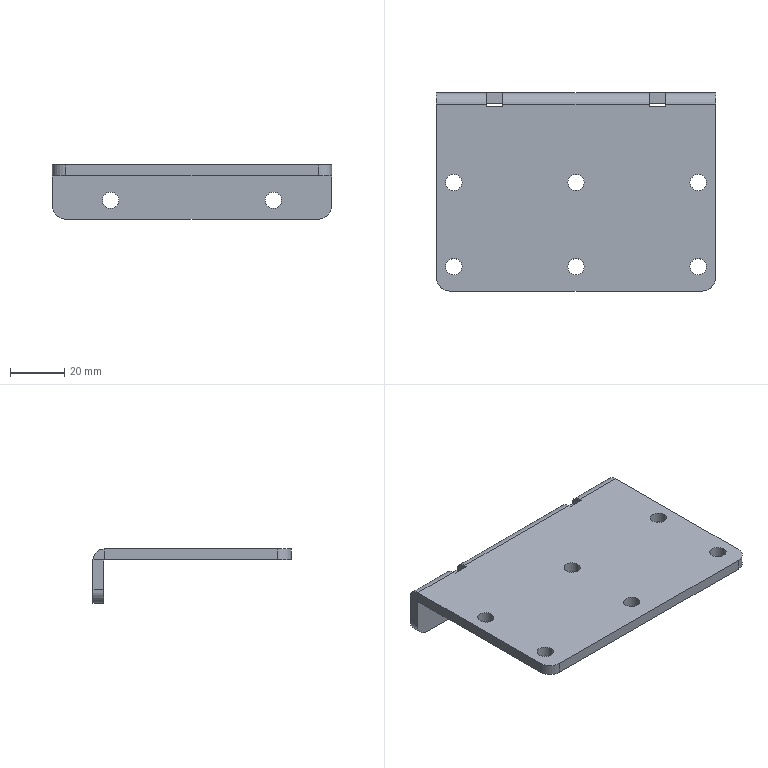Part | SolidWorks | features ICE 3, EdgeFlange 1, Fillet 1, FlatPattern 1, SMBaseFlange 1, SheetMetal 1 | 1 solid | 48 faces | box 103 x 73 x 20 mm | volume 35104 mm3 | cylinder 26 | plane 22 | commonest cylinder face diameters 6 x16 10 x4 0.2 x3 8.2 x3
STEP:
#1=CARTESIAN_POINT('',(-3.,3.5,-4.));
#2=VERTEX_POINT('',#1);
#3=CARTESIAN_POINT('',(3.,3.5,-4.));
#4=VERTEX_POINT('',#3);
#5=CARTESIAN_POINT('',(0.,3.5,-4.));
#6=DIRECTION('',(0.,0.,1.));
#7=DIRECTION('',(1.,0.,0.));
#8=AXIS2_PLACEMENT_3D('',#5,#6,#7);
#9=CIRCLE('',#8,3.);
#10=EDGE_CURVE('',#2,#4,#9,.T.);
#11=ORIENTED_EDGE('',*,*,#10,.F.);
#12=CARTESIAN_POINT('',(-3.,3.5,0.));
#13=VERTEX_POINT('',#12);
#14=CARTESIAN_POINT('',(-3.,3.5,-10.));
#15=DIRECTION('',(0.,0.,1.));
#16=VECTOR('',#15,1000.);
#17=LINE('',#14,#16);
#18=EDGE_CURVE('',#2,#13,#17,.T.);
#19=ORIENTED_EDGE('',*,*,#18,.T.);
#20=CARTESIAN_POINT('',(3.,3.5,0.));
#21=VERTEX_POINT('',#20);
#22=CARTESIAN_POINT('',(0.,3.5,0.));
#23=DIRECTION('',(0.,0.,1.));
#24=DIRECTION('',(1.,0.,0.));
#25=AXIS2_PLACEMENT_3D('',#22,#23,#24);
#26=CIRCLE('',#25,3.);
#27=EDGE_CURVE('',#13,#21,#26,.T.);
#28=ORIENTED_EDGE('',*,*,#27,.T.);
#29=CARTESIAN_POINT('',(3.,3.5,-10.));
#30=DIRECTION('',(0.,0.,1.));
#31=VECTOR('',#30,1000.);
#32=LINE('',#29,#31);
#33=EDGE_CURVE('',#4,#21,#32,.T.);
#34=ORIENTED_EDGE('',*,*,#33,.F.);
#35=EDGE_LOOP('',(#11,#19,#28,#34));
#36=FACE_OUTER_BOUND('',#35,.T.);
#37=CARTESIAN_POINT('',(0.,3.5,-10.));
#38=DIRECTION('',(0.,0.,1.));
#39=DIRECTION('',(1.,0.,0.));
#40=AXIS2_PLACEMENT_3D('',#37,#38,#39);
#41=CYLINDRICAL_SURFACE('',#40,3.);
#42=ADVANCED_FACE('',(#36),#41,.F.);
#43=CARTESIAN_POINT('',(42.,3.5,-4.));
#44=VERTEX_POINT('',#43);
#45=CARTESIAN_POINT('',(48.,3.5,-4.));
#46=VERTEX_POINT('',#45);
#47=CARTESIAN_POINT('',(45.,3.5,-4.));
#48=DIRECTION('',(0.,0.,1.));
#49=DIRECTION('',(1.,0.,0.));
#50=AXIS2_PLACEMENT_3D('',#47,#48,#49);
#51=CIRCLE('',#50,3.);
#52=EDGE_CURVE('',#44,#46,#51,.T.);
#53=ORIENTED_EDGE('',*,*,#52,.F.);
#54=CARTESIAN_POINT('',(42.,3.5,0.));
#55=VERTEX_POINT('',#54);
#56=CARTESIAN_POINT('',(42.,3.5,-10.));
#57=DIRECTION('',(0.,0.,1.));
#58=VECTOR('',#57,1000.);
#59=LINE('',#56,#58);
#60=EDGE_CURVE('',#44,#55,#59,.T.);
#61=ORIENTED_EDGE('',*,*,#60,.T.);
#62=CARTESIAN_POINT('',(48.,3.5,0.));
#63=VERTEX_POINT('',#62);
#64=CARTESIAN_POINT('',(45.,3.5,0.));
#65=DIRECTION('',(0.,0.,1.));
#66=DIRECTION('',(-1.,0.,0.));
#67=AXIS2_PLACEMENT_3D('',#64,#65,#66);
#68=CIRCLE('',#67,3.);
#69=EDGE_CURVE('',#55,#63,#68,.T.);
#70=ORIENTED_EDGE('',*,*,#69,.T.);
#71=CARTESIAN_POINT('',(48.,3.5,-10.));
#72=DIRECTION('',(0.,0.,1.));
#73=VECTOR('',#72,1000.);
#74=LINE('',#71,#73);
#75=EDGE_CURVE('',#46,#63,#74,.T.);
#76=ORIENTED_EDGE('',*,*,#75,.F.);
#77=EDGE_LOOP('',(#53,#61,#70,#76));
#78=FACE_OUTER_BOUND('',#77,.T.);
#79=CARTESIAN_POINT('',(45.,3.5,-10.));
#80=DIRECTION('',(0.,0.,1.));
#81=DIRECTION('',(1.,0.,0.));
#82=AXIS2_PLACEMENT_3D('',#79,#80,#81);
#83=CYLINDRICAL_SURFACE('',#82,3.);
#84=ADVANCED_FACE('',(#78),#83,.F.);
#85=CARTESIAN_POINT('',(42.,-27.5,-4.));
#86=VERTEX_POINT('',#85);
#87=CARTESIAN_POINT('',(48.,-27.5,-4.));
#88=VERTEX_POINT('',#87);
#89=CARTESIAN_POINT('',(45.,-27.5,-4.));
#90=DIRECTION('',(0.,0.,1.));
#91=DIRECTION('',(1.,0.,0.));
#92=AXIS2_PLACEMENT_3D('',#89,#90,#91);
#93=CIRCLE('',#92,3.);
#94=EDGE_CURVE('',#86,#88,#93,.T.);
#95=ORIENTED_EDGE('',*,*,#94,.F.);
#96=CARTESIAN_POINT('',(42.,-27.5,0.));
#97=VERTEX_POINT('',#96);
#98=CARTESIAN_POINT('',(42.,-27.5,-10.));
#99=DIRECTION('',(0.,0.,1.));
#100=VECTOR('',#99,1000.);
#101=LINE('',#98,#100);
#102=EDGE_CURVE('',#86,#97,#101,.T.);
#103=ORIENTED_EDGE('',*,*,#102,.T.);
#104=CARTESIAN_POINT('',(48.,-27.5,0.));
#105=VERTEX_POINT('',#104);
#106=CARTESIAN_POINT('',(45.,-27.5,0.));
#107=DIRECTION('',(0.,0.,1.));
#108=DIRECTION('',(-1.,0.,0.));
#109=AXIS2_PLACEMENT_3D('',#106,#107,#108);
#110=CIRCLE('',#109,3.);
#111=EDGE_CURVE('',#97,#105,#110,.T.);
#112=ORIENTED_EDGE('',*,*,#111,.T.);
#113=CARTESIAN_POINT('',(48.,-27.5,-10.));
#114=DIRECTION('',(0.,0.,1.));
#115=VECTOR('',#114,1000.);
#116=LINE('',#113,#115);
#117=EDGE_CURVE('',#88,#105,#116,.T.);
#118=ORIENTED_EDGE('',*,*,#117,.F.);
#119=EDGE_LOOP('',(#95,#103,#112,#118));
#120=FACE_OUTER_BOUND('',#119,.T.);
#121=CARTESIAN_POINT('',(45.,-27.5,-10.));
#122=DIRECTION('',(0.,0.,1.));
#123=DIRECTION('',(1.,0.,0.));
#124=AXIS2_PLACEMENT_3D('',#121,#122,#123);
#125=CYLINDRICAL_SURFACE('',#124,3.);
#126=ADVANCED_FACE('',(#120),#125,.F.);
#127=CARTESIAN_POINT('',(-48.,3.5,-4.));
#128=VERTEX_POINT('',#127);
#129=CARTESIAN_POINT('',(-42.,3.5,-4.));
#130=VERTEX_POINT('',#129);
#131=CARTESIAN_POINT('',(-45.,3.5,-4.));
#132=DIRECTION('',(0.,0.,1.));
#133=DIRECTION('',(1.,0.,0.));
#134=AXIS2_PLACEMENT_3D('',#131,#132,#133);
#135=CIRCLE('',#134,3.);
#136=EDGE_CURVE('',#128,#130,#135,.T.);
#137=ORIENTED_EDGE('',*,*,#136,.F.);
#138=CARTESIAN_POINT('',(-48.,3.5,0.));
#139=VERTEX_POINT('',#138);
#140=CARTESIAN_POINT('',(-48.,3.5,-10.));
#141=DIRECTION('',(0.,0.,1.));
#142=VECTOR('',#141,1000.);
#143=LINE('',#140,#142);
#144=EDGE_CURVE('',#128,#139,#143,.T.);
#145=ORIENTED_EDGE('',*,*,#144,.T.);
#146=CARTESIAN_POINT('',(-42.,3.5,0.));
#147=VERTEX_POINT('',#146);
#148=CARTESIAN_POINT('',(-45.,3.5,0.));
#149=DIRECTION('',(0.,0.,1.));
#150=DIRECTION('',(1.,0.,0.));
#151=AXIS2_PLACEMENT_3D('',#148,#149,#150);
#152=CIRCLE('',#151,3.);
#153=EDGE_CURVE('',#139,#147,#152,.T.);
#154=ORIENTED_EDGE('',*,*,#153,.T.);
#155=CARTESIAN_POINT('',(-42.,3.5,-10.));
#156=DIRECTION('',(0.,0.,1.));
#157=VECTOR('',#156,1000.);
#158=LINE('',#155,#157);
#159=EDGE_CURVE('',#130,#147,#158,.T.);
#160=ORIENTED_EDGE('',*,*,#159,.F.);
#161=EDGE_LOOP('',(#137,#145,#154,#160));
#162=FACE_OUTER_BOUND('',#161,.T.);
#163=CARTESIAN_POINT('',(-45.,3.5,-10.));
#164=DIRECTION('',(0.,0.,1.));
#165=DIRECTION('',(1.,0.,0.));
#166=AXIS2_PLACEMENT_3D('',#163,#164,#165);
#167=CYLINDRICAL_SURFACE('',#166,3.);
#168=ADVANCED_FACE('',(#162),#167,.F.);
#169=CARTESIAN_POINT('',(-3.,-27.5,-4.));
#170=VERTEX_POINT('',#169);
#171=CARTESIAN_POINT('',(3.,-27.5,-4.));
#172=VERTEX_POINT('',#171);
#173=CARTESIAN_POINT('',(0.,-27.5,-4.));
#174=DIRECTION('',(0.,0.,1.));
#175=DIRECTION('',(1.,0.,0.));
#176=AXIS2_PLACEMENT_3D('',#173,#174,#175);
#177=CIRCLE('',#176,3.);
#178=EDGE_CURVE('',#170,#172,#177,.T.);
#179=ORIENTED_EDGE('',*,*,#178,.F.);
#180=CARTESIAN_POINT('',(-3.,-27.5,0.));
#181=VERTEX_POINT('',#180);
#182=CARTESIAN_POINT('',(-3.,-27.5,-10.));
#183=DIRECTION('',(0.,0.,1.));
#184=VECTOR('',#183,1000.);
#185=LINE('',#182,#184);
#186=EDGE_CURVE('',#170,#181,#185,.T.);
#187=ORIENTED_EDGE('',*,*,#186,.T.);
#188=CARTESIAN_POINT('',(3.,-27.5,0.));
#189=VERTEX_POINT('',#188);
#190=CARTESIAN_POINT('',(0.,-27.5,0.));
#191=DIRECTION('',(0.,0.,1.));
#192=DIRECTION('',(1.,0.,0.));
#193=AXIS2_PLACEMENT_3D('',#190,#191,#192);
#194=CIRCLE('',#193,3.);
#195=EDGE_CURVE('',#181,#189,#194,.T.);
#196=ORIENTED_EDGE('',*,*,#195,.T.);
#197=CARTESIAN_POINT('',(3.,-27.5,-10.));
#198=DIRECTION('',(0.,0.,1.));
#199=VECTOR('',#198,1000.);
#200=LINE('',#197,#199);
#201=EDGE_CURVE('',#172,#189,#200,.T.);
#202=ORIENTED_EDGE('',*,*,#201,.F.);
#203=EDGE_LOOP('',(#179,#187,#196,#202));
#204=FACE_OUTER_BOUND('',#203,.T.);
#205=CARTESIAN_POINT('',(0.,-27.5,-10.));
#206=DIRECTION('',(0.,0.,1.));
#207=DIRECTION('',(1.,0.,0.));
#208=AXIS2_PLACEMENT_3D('',#205,#206,#207);
#209=CYLINDRICAL_SURFACE('',#208,3.);
#210=ADVANCED_FACE('',(#204),#209,.F.);
#211=CARTESIAN_POINT('',(-48.,-27.5,-4.));
#212=VERTEX_POINT('',#211);
#213=CARTESIAN_POINT('',(-42.,-27.5,-4.));
#214=VERTEX_POINT('',#213);
#215=CARTESIAN_POINT('',(-45.,-27.5,-4.));
#216=DIRECTION('',(0.,0.,1.));
#217=DIRECTION('',(1.,0.,0.));
#218=AXIS2_PLACEMENT_3D('',#215,#216,#217);
#219=CIRCLE('',#218,3.);
#220=EDGE_CURVE('',#212,#214,#219,.T.);
#221=ORIENTED_EDGE('',*,*,#220,.F.);
#222=CARTESIAN_POINT('',(-48.,-27.5,0.));
#223=VERTEX_POINT('',#222);
#224=CARTESIAN_POINT('',(-48.,-27.5,-10.));
#225=DIRECTION('',(0.,0.,1.));
#226=VECTOR('',#225,1000.);
#227=LINE('',#224,#226);
#228=EDGE_CURVE('',#212,#223,#227,.T.);
#229=ORIENTED_EDGE('',*,*,#228,.T.);
#230=CARTESIAN_POINT('',(-42.,-27.5,0.));
#231=VERTEX_POINT('',#230);
#232=CARTESIAN_POINT('',(-45.,-27.5,0.));
#233=DIRECTION('',(0.,0.,1.));
#234=DIRECTION('',(1.,0.,0.));
#235=AXIS2_PLACEMENT_3D('',#232,#233,#234);
#236=CIRCLE('',#235,3.);
#237=EDGE_CURVE('',#223,#231,#236,.T.);
#238=ORIENTED_EDGE('',*,*,#237,.T.);
#239=CARTESIAN_POINT('',(-42.,-27.5,-10.));
#240=DIRECTION('',(0.,0.,1.));
#241=VECTOR('',#240,1000.);
#242=LINE('',#239,#241);
#243=EDGE_CURVE('',#214,#231,#242,.T.);
#244=ORIENTED_EDGE('',*,*,#243,.F.);
#245=EDGE_LOOP('',(#221,#229,#238,#244));
#246=FACE_OUTER_BOUND('',#245,.T.);
#247=CARTESIAN_POINT('',(-45.,-27.5,-10.));
#248=DIRECTION('',(0.,0.,1.));
#249=DIRECTION('',(1.,0.,0.));
#250=AXIS2_PLACEMENT_3D('',#247,#248,#249);
#251=CYLINDRICAL_SURFACE('',#250,3.);
#252=ADVANCED_FACE('',(#246),#251,.F.);
#253=CARTESIAN_POINT('',(-30.,32.5,-16.));
#254=VERTEX_POINT('',#253);
#255=CARTESIAN_POINT('',(-30.,32.5,-10.));
#256=VERTEX_POINT('',#255);
#257=CARTESIAN_POINT('',(-30.,32.5,-13.));
#258=DIRECTION('',(0.,1.,0.));
#259=DIRECTION('',(0.,0.,1.));
#260=AXIS2_PLACEMENT_3D('',#257,#258,#259);
#261=CIRCLE('',#260,3.);
#262=EDGE_CURVE('',#254,#256,#261,.T.);
#263=ORIENTED_EDGE('',*,*,#262,.F.);
#264=CARTESIAN_POINT('',(-30.,36.5,-16.));
#265=VERTEX_POINT('',#264);
#266=CARTESIAN_POINT('',(-30.,26.5,-16.));
#267=DIRECTION('',(0.,1.,0.));
#268=VECTOR('',#267,1000.);
#269=LINE('',#266,#268);
#270=EDGE_CURVE('',#254,#265,#269,.T.);
#271=ORIENTED_EDGE('',*,*,#270,.T.);
#272=CARTESIAN_POINT('',(-30.,36.5,-10.));
#273=VERTEX_POINT('',#272);
#274=CARTESIAN_POINT('',(-30.,36.5,-13.));
#275=DIRECTION('',(0.,1.,0.));
#276=DIRECTION('',(0.,0.,1.));
#277=AXIS2_PLACEMENT_3D('',#274,#275,#276);
#278=CIRCLE('',#277,3.);
#279=EDGE_CURVE('',#265,#273,#278,.T.);
#280=ORIENTED_EDGE('',*,*,#279,.T.);
#281=CARTESIAN_POINT('',(-30.,26.5,-10.));
#282=DIRECTION('',(0.,1.,0.));
#283=VECTOR('',#282,1000.);
#284=LINE('',#281,#283);
#285=EDGE_CURVE('',#256,#273,#284,.T.);
#286=ORIENTED_EDGE('',*,*,#285,.F.);
#287=EDGE_LOOP('',(#263,#271,#280,#286));
#288=FACE_OUTER_BOUND('',#287,.T.);
#289=CARTESIAN_POINT('',(-30.,26.5,-13.));
#290=DIRECTION('',(0.,1.,0.));
#291=DIRECTION('',(0.,0.,1.));
#292=AXIS2_PLACEMENT_3D('',#289,#290,#291);
#293=CYLINDRICAL_SURFACE('',#292,3.);
#294=ADVANCED_FACE('',(#288),#293,.F.);
#295=CARTESIAN_POINT('',(30.,32.5,-16.));
#296=VERTEX_POINT('',#295);
#297=CARTESIAN_POINT('',(30.,32.5,-10.));
#298=VERTEX_POINT('',#297);
#299=CARTESIAN_POINT('',(30.,32.5,-13.));
#300=DIRECTION('',(0.,1.,0.));
#301=DIRECTION('',(0.,0.,1.));
#302=AXIS2_PLACEMENT_3D('',#299,#300,#301);
#303=CIRCLE('',#302,3.);
#304=EDGE_CURVE('',#296,#298,#303,.T.);
#305=ORIENTED_EDGE('',*,*,#304,.F.);
#306=CARTESIAN_POINT('',(30.,36.5,-16.));
#307=VERTEX_POINT('',#306);
#308=CARTESIAN_POINT('',(30.,26.5,-16.));
#309=DIRECTION('',(0.,1.,0.));
#310=VECTOR('',#309,1000.);
#311=LINE('',#308,#310);
#312=EDGE_CURVE('',#296,#307,#311,.T.);
#313=ORIENTED_EDGE('',*,*,#312,.T.);
#314=CARTESIAN_POINT('',(30.,36.5,-10.));
#315=VERTEX_POINT('',#314);
#316=CARTESIAN_POINT('',(30.,36.5,-13.));
#317=DIRECTION('',(0.,1.,0.));
#318=DIRECTION('',(0.,0.,-1.));
#319=AXIS2_PLACEMENT_3D('',#316,#317,#318);
#320=CIRCLE('',#319,3.);
#321=EDGE_CURVE('',#307,#315,#320,.T.);
#322=ORIENTED_EDGE('',*,*,#321,.T.);
#323=CARTESIAN_POINT('',(30.,26.5,-10.));
#324=DIRECTION('',(0.,1.,0.));
#325=VECTOR('',#324,1000.);
#326=LINE('',#323,#325);
#327=EDGE_CURVE('',#298,#315,#326,.T.);
#328=ORIENTED_EDGE('',*,*,#327,.F.);
#329=EDGE_LOOP('',(#305,#313,#322,#328));
#330=FACE_OUTER_BOUND('',#329,.T.);
#331=CARTESIAN_POINT('',(30.,26.5,-13.));
#332=DIRECTION('',(0.,1.,0.));
#333=DIRECTION('',(0.,0.,1.));
#334=AXIS2_PLACEMENT_3D('',#331,#332,#333);
#335=CYLINDRICAL_SURFACE('',#334,3.);
#336=ADVANCED_FACE('',(#330),#335,.F.);
#337=CARTESIAN_POINT('',(-27.,31.5,0.));
#338=VERTEX_POINT('',#337);
#339=CARTESIAN_POINT('',(-27.,32.4,0.));
#340=VERTEX_POINT('',#339);
#341=CARTESIAN_POINT('',(-27.,31.5,0.));
#342=DIRECTION('',(0.,1.,0.));
#343=VECTOR('',#342,1000.);
#344=LINE('',#341,#343);
#345=EDGE_CURVE('',#338,#340,#344,.T.);
#346=ORIENTED_EDGE('',*,*,#345,.T.);
#347=CARTESIAN_POINT('',(-27.,32.4,-4.));
#348=VERTEX_POINT('',#347);
#349=CARTESIAN_POINT('',(-27.,32.4,0.));
#350=DIRECTION('',(0.,0.,-1.));
#351=VECTOR('',#350,1000.);
#352=LINE('',#349,#351);
#353=EDGE_CURVE('',#340,#348,#352,.T.);
#354=ORIENTED_EDGE('',*,*,#353,.T.);
#355=CARTESIAN_POINT('',(-27.,31.5,-4.));
#356=VERTEX_POINT('',#355);
#357=CARTESIAN_POINT('',(-27.,0.,-4.));
#358=DIRECTION('',(0.,1.,0.));
#359=VECTOR('',#358,1000.);
#360=LINE('',#357,#359);
#361=EDGE_CURVE('',#356,#348,#360,.T.);
#362=ORIENTED_EDGE('',*,*,#361,.F.);
#363=CARTESIAN_POINT('',(-27.,31.5,-4.1));
#364=DIRECTION('',(0.,0.,-1.));
#365=VECTOR('',#364,1000.);
#366=LINE('',#363,#365);
#367=EDGE_CURVE('',#338,#356,#366,.T.);
#368=ORIENTED_EDGE('',*,*,#367,.F.);
#369=EDGE_LOOP('',(#346,#354,#362,#368));
#370=FACE_OUTER_BOUND('',#369,.T.);
#371=CARTESIAN_POINT('',(-27.,31.5,-4.1));
#372=DIRECTION('',(1.,0.,0.));
#373=DIRECTION('',(0.,0.,-1.));
#374=AXIS2_PLACEMENT_3D('',#371,#372,#373);
#375=PLANE('',#374);
#376=ADVANCED_FACE('',(#370),#375,.F.);
#377=CARTESIAN_POINT('',(33.,31.5,0.));
#378=VERTEX_POINT('',#377);
#379=CARTESIAN_POINT('',(33.,32.4,0.));
#380=VERTEX_POINT('',#379);
#381=CARTESIAN_POINT('',(33.,31.5,0.));
#382=DIRECTION('',(0.,1.,0.));
#383=VECTOR('',#382,1000.);
#384=LINE('',#381,#383);
#385=EDGE_CURVE('',#378,#380,#384,.T.);
#386=ORIENTED_EDGE('',*,*,#385,.T.);
#387=CARTESIAN_POINT('',(33.,32.4,-4.));
#388=VERTEX_POINT('',#387);
#389=CARTESIAN_POINT('',(33.,32.4,0.));
#390=DIRECTION('',(0.,0.,-1.));
#391=VECTOR('',#390,1000.);
#392=LINE('',#389,#391);
#393=EDGE_CURVE('',#380,#388,#392,.T.);
#394=ORIENTED_EDGE('',*,*,#393,.T.);
#395=CARTESIAN_POINT('',(33.,31.5,-4.));
#396=VERTEX_POINT('',#395);
#397=CARTESIAN_POINT('',(33.,0.,-4.));
#398=DIRECTION('',(0.,1.,0.));
#399=VECTOR('',#398,1000.);
#400=LINE('',#397,#399);
#401=EDGE_CURVE('',#396,#388,#400,.T.);
#402=ORIENTED_EDGE('',*,*,#401,.F.);
#403=CARTESIAN_POINT('',(33.,31.5,-4.1));
#404=DIRECTION('',(0.,0.,-1.));
#405=VECTOR('',#404,1000.);
#406=LINE('',#403,#405);
#407=EDGE_CURVE('',#378,#396,#406,.T.);
#408=ORIENTED_EDGE('',*,*,#407,.F.);
#409=EDGE_LOOP('',(#386,#394,#402,#408));
#410=FACE_OUTER_BOUND('',#409,.T.);
#411=CARTESIAN_POINT('',(33.,31.5,-4.1));
#412=DIRECTION('',(1.,0.,0.));
#413=DIRECTION('',(0.,1.,0.));
#414=AXIS2_PLACEMENT_3D('',#411,#412,#413);
#415=PLANE('',#414);
#416=ADVANCED_FACE('',(#410),#415,.F.);
#417=CARTESIAN_POINT('',(-33.,36.5,-4.1));
#418=VERTEX_POINT('',#417);
#419=CARTESIAN_POINT('',(-33.,32.4,0.));
#420=VERTEX_POINT('',#419);
#421=CARTESIAN_POINT('',(-33.,32.4,-4.1));
#422=DIRECTION('',(1.,0.,0.));
#423=DIRECTION('',(0.,-1.,0.));
#424=AXIS2_PLACEMENT_3D('',#421,#422,#423);
#425=CIRCLE('',#424,4.1);
#426=EDGE_CURVE('',#418,#420,#425,.T.);
#427=ORIENTED_EDGE('',*,*,#426,.F.);
#428=CARTESIAN_POINT('',(-51.5,36.5,-4.1));
#429=VERTEX_POINT('',#428);
#430=CARTESIAN_POINT('',(0.,36.5,-4.1));
#431=DIRECTION('',(1.,0.,0.));
#432=VECTOR('',#431,1000.);
#433=LINE('',#430,#432);
#434=EDGE_CURVE('',#429,#418,#433,.T.);
#435=ORIENTED_EDGE('',*,*,#434,.F.);
#436=CARTESIAN_POINT('',(-51.5,32.4,0.));
#437=VERTEX_POINT('',#436);
#438=CARTESIAN_POINT('',(-51.5,32.4,-4.1));
#439=DIRECTION('',(-1.,0.,0.));
#440=DIRECTION('',(0.,0.,-1.));
#441=AXIS2_PLACEMENT_3D('',#438,#439,#440);
#442=CIRCLE('',#441,4.1);
#443=EDGE_CURVE('',#437,#429,#442,.T.);
#444=ORIENTED_EDGE('',*,*,#443,.F.);
#445=CARTESIAN_POINT('',(51.5,32.4,0.));
#446=DIRECTION('',(-1.,0.,0.));
#447=VECTOR('',#446,1000.);
#448=LINE('',#445,#447);
#449=EDGE_CURVE('',#420,#437,#448,.T.);
#450=ORIENTED_EDGE('',*,*,#449,.F.);
#451=EDGE_LOOP('',(#427,#435,#444,#450));
#452=FACE_OUTER_BOUND('',#451,.T.);
#453=CARTESIAN_POINT('',(51.5,32.4,-4.1));
#454=DIRECTION('',(1.,0.,0.));
#455=DIRECTION('',(0.,1.,0.));
#456=AXIS2_PLACEMENT_3D('',#453,#454,#455);
#457=CYLINDRICAL_SURFACE('',#456,4.1);
#458=ADVANCED_FACE('',(#452),#457,.T.);
#459=CARTESIAN_POINT('',(-27.,36.5,-4.1));
#460=VERTEX_POINT('',#459);
#461=CARTESIAN_POINT('',(-27.,32.4,-4.1));
#462=DIRECTION('',(-1.,0.,0.));
#463=DIRECTION('',(0.,0.,-1.));
#464=AXIS2_PLACEMENT_3D('',#461,#462,#463);
#465=CIRCLE('',#464,4.1);
#466=EDGE_CURVE('',#340,#460,#465,.T.);
#467=ORIENTED_EDGE('',*,*,#466,.F.);
#468=CARTESIAN_POINT('',(27.,32.4,0.));
#469=VERTEX_POINT('',#468);
#470=CARTESIAN_POINT('',(51.5,32.4,0.));
#471=DIRECTION('',(-1.,0.,0.));
#472=VECTOR('',#471,1000.);
#473=LINE('',#470,#472);
#474=EDGE_CURVE('',#469,#340,#473,.T.);
#475=ORIENTED_EDGE('',*,*,#474,.F.);
#476=CARTESIAN_POINT('',(27.,36.5,-4.1));
#477=VERTEX_POINT('',#476);
#478=CARTESIAN_POINT('',(27.,32.4,-4.1));
#479=DIRECTION('',(1.,0.,0.));
#480=DIRECTION('',(0.,0.,1.));
#481=AXIS2_PLACEMENT_3D('',#478,#479,#480);
#482=CIRCLE('',#481,4.1);
#483=EDGE_CURVE('',#477,#469,#482,.T.);
#484=ORIENTED_EDGE('',*,*,#483,.F.);
#485=CARTESIAN_POINT('',(0.,36.5,-4.1));
#486=DIRECTION('',(1.,0.,0.));
#487=VECTOR('',#486,1000.);
#488=LINE('',#485,#487);
#489=EDGE_CURVE('',#460,#477,#488,.T.);
#490=ORIENTED_EDGE('',*,*,#489,.F.);
#491=EDGE_LOOP('',(#467,#475,#484,#490));
#492=FACE_OUTER_BOUND('',#491,.T.);
#493=CARTESIAN_POINT('',(51.5,32.4,-4.1));
#494=DIRECTION('',(1.,0.,0.));
#495=DIRECTION('',(0.,1.,0.));
#496=AXIS2_PLACEMENT_3D('',#493,#494,#495);
#497=CYLINDRICAL_SURFACE('',#496,4.1);
#498=ADVANCED_FACE('',(#492),#497,.T.);
#499=CARTESIAN_POINT('',(-51.5,32.5,-4.1));
#500=VERTEX_POINT('',#499);
#501=CARTESIAN_POINT('',(-33.,32.5,-4.1));
#502=VERTEX_POINT('',#501);
#503=CARTESIAN_POINT('',(-51.5,32.5,-4.1));
#504=DIRECTION('',(1.,0.,0.));
#505=VECTOR('',#504,1000.);
#506=LINE('',#503,#505);
#507=EDGE_CURVE('',#500,#502,#506,.T.);
#508=ORIENTED_EDGE('',*,*,#507,.T.);
#509=CARTESIAN_POINT('',(-33.,32.4,-4.));
#510=VERTEX_POINT('',#509);
#511=CARTESIAN_POINT('',(-33.,32.4,-4.1));
#512=DIRECTION('',(1.,0.,0.));
#513=DIRECTION('',(0.,-1.,0.));
#514=AXIS2_PLACEMENT_3D('',#511,#512,#513);
#515=CIRCLE('',#514,0.1);
#516=EDGE_CURVE('',#502,#510,#515,.T.);
#517=ORIENTED_EDGE('',*,*,#516,.T.);
#518=CARTESIAN_POINT('',(-51.5,32.4,-4.));
#519=VERTEX_POINT('',#518);
#520=CARTESIAN_POINT('',(51.5,32.4,-4.));
#521=DIRECTION('',(-1.,0.,0.));
#522=VECTOR('',#521,1000.);
#523=LINE('',#520,#522);
#524=EDGE_CURVE('',#510,#519,#523,.T.);
#525=ORIENTED_EDGE('',*,*,#524,.T.);
#526=CARTESIAN_POINT('',(-51.5,32.4,-4.1));
#527=DIRECTION('',(-1.,0.,0.));
#528=DIRECTION('',(0.,0.,-1.));
#529=AXIS2_PLACEMENT_3D('',#526,#527,#528);
#530=CIRCLE('',#529,0.1);
#531=EDGE_CURVE('',#519,#500,#530,.T.);
#532=ORIENTED_EDGE('',*,*,#531,.T.);
#533=EDGE_LOOP('',(#508,#517,#525,#532));
#534=FACE_OUTER_BOUND('',#533,.T.);
#535=CARTESIAN_POINT('',(51.5,32.4,-4.1));
#536=DIRECTION('',(1.,0.,0.));
#537=DIRECTION('',(0.,1.,0.));
#538=AXIS2_PLACEMENT_3D('',#535,#536,#537);
#539=CYLINDRICAL_SURFACE('',#538,0.1);
#540=ADVANCED_FACE('',(#534),#539,.F.);
#541=CARTESIAN_POINT('',(27.,32.4,-4.));
#542=VERTEX_POINT('',#541);
#543=CARTESIAN_POINT('',(51.5,32.4,-4.));
#544=DIRECTION('',(-1.,0.,0.));
#545=VECTOR('',#544,1000.);
#546=LINE('',#543,#545);
#547=EDGE_CURVE('',#542,#348,#546,.T.);
#548=ORIENTED_EDGE('',*,*,#547,.T.);
#549=CARTESIAN_POINT('',(-27.,32.5,-4.1));
#550=VERTEX_POINT('',#549);
#551=CARTESIAN_POINT('',(-27.,32.4,-4.1));
#552=DIRECTION('',(-1.,0.,0.));
#553=DIRECTION('',(0.,0.,-1.));
#554=AXIS2_PLACEMENT_3D('',#551,#552,#553);
#555=CIRCLE('',#554,0.1);
#556=EDGE_CURVE('',#348,#550,#555,.T.);
#557=ORIENTED_EDGE('',*,*,#556,.T.);
#558=CARTESIAN_POINT('',(27.,32.5,-4.1));
#559=VERTEX_POINT('',#558);
#560=CARTESIAN_POINT('',(-51.5,32.5,-4.1));
#561=DIRECTION('',(1.,0.,0.));
#562=VECTOR('',#561,1000.);
#563=LINE('',#560,#562);
#564=EDGE_CURVE('',#550,#559,#563,.T.);
#565=ORIENTED_EDGE('',*,*,#564,.T.);
#566=CARTESIAN_POINT('',(27.,32.4,-4.1));
#567=DIRECTION('',(1.,0.,0.));
#568=DIRECTION('',(0.,0.,1.));
#569=AXIS2_PLACEMENT_3D('',#566,#567,#568);
#570=CIRCLE('',#569,0.1);
#571=EDGE_CURVE('',#559,#542,#570,.T.);
#572=ORIENTED_EDGE('',*,*,#571,.T.);
#573=EDGE_LOOP('',(#548,#557,#565,#572));
#574=FACE_OUTER_BOUND('',#573,.T.);
#575=CARTESIAN_POINT('',(51.5,32.4,-4.1));
#576=DIRECTION('',(1.,0.,0.));
#577=DIRECTION('',(0.,1.,0.));
#578=AXIS2_PLACEMENT_3D('',#575,#576,#577);
#579=CYLINDRICAL_SURFACE('',#578,0.1);
#580=ADVANCED_FACE('',(#574),#579,.F.);
#581=CARTESIAN_POINT('',(51.5,-31.5,0.));
#582=VERTEX_POINT('',#581);
#583=CARTESIAN_POINT('',(51.5,32.4,0.));
#584=VERTEX_POINT('',#583);
#585=CARTESIAN_POINT('',(51.5,-36.5,0.));
#586=DIRECTION('',(0.,1.,0.));
#587=VECTOR('',#586,1000.);
#588=LINE('',#585,#587);
#589=EDGE_CURVE('',#582,#584,#588,.T.);
#590=ORIENTED_EDGE('',*,*,#589,.F.);
#591=CARTESIAN_POINT('',(51.5,-31.5,-4.));
#592=VERTEX_POINT('',#591);
#593=CARTESIAN_POINT('',(51.5,-31.5,-4.));
#594=DIRECTION('',(0.,0.,-1.));
#595=VECTOR('',#594,1000.);
#596=LINE('',#593,#595);
#597=EDGE_CURVE('',#582,#592,#596,.T.);
#598=ORIENTED_EDGE('',*,*,#597,.T.);
#599=CARTESIAN_POINT('',(51.5,32.4,-4.));
#600=VERTEX_POINT('',#599);
#601=CARTESIAN_POINT('',(51.5,-36.5,-4.));
#602=DIRECTION('',(0.,1.,0.));
#603=VECTOR('',#602,1000.);
#604=LINE('',#601,#603);
#605=EDGE_CURVE('',#592,#600,#604,.T.);
#606=ORIENTED_EDGE('',*,*,#605,.T.);
#607=CARTESIAN_POINT('',(51.5,32.4,-4.));
#608=DIRECTION('',(0.,0.,1.));
#609=VECTOR('',#608,1000.);
#610=LINE('',#607,#609);
#611=EDGE_CURVE('',#600,#584,#610,.T.);
#612=ORIENTED_EDGE('',*,*,#611,.T.);
#613=EDGE_LOOP('',(#590,#598,#606,#612));
#614=FACE_OUTER_BOUND('',#613,.T.);
#615=CARTESIAN_POINT('',(51.5,-36.5,-4.));
#616=DIRECTION('',(1.,0.,0.));
#617=DIRECTION('',(0.,0.,-1.));
#618=AXIS2_PLACEMENT_3D('',#615,#616,#617);
#619=PLANE('',#618);
#620=ADVANCED_FACE('',(#614),#619,.T.);
#621=ORIENTED_EDGE('',*,*,#524,.F.);
#622=CARTESIAN_POINT('',(-33.,31.5,-4.));
#623=VERTEX_POINT('',#622);
#624=CARTESIAN_POINT('',(-33.,0.,-4.));
#625=DIRECTION('',(0.,-1.,0.));
#626=VECTOR('',#625,1000.);
#627=LINE('',#624,#626);
#628=EDGE_CURVE('',#510,#623,#627,.T.);
#629=ORIENTED_EDGE('',*,*,#628,.T.);
#630=CARTESIAN_POINT('',(0.,31.5,-4.));
#631=DIRECTION('',(-1.,0.,0.));
#632=VECTOR('',#631,1000.);
#633=LINE('',#630,#632);
#634=EDGE_CURVE('',#356,#623,#633,.T.);
#635=ORIENTED_EDGE('',*,*,#634,.F.);
#636=ORIENTED_EDGE('',*,*,#361,.T.);
#637=ORIENTED_EDGE('',*,*,#547,.F.);
#638=CARTESIAN_POINT('',(27.,31.5,-4.));
#639=VERTEX_POINT('',#638);
#640=CARTESIAN_POINT('',(27.,0.,-4.));
#641=DIRECTION('',(0.,-1.,0.));
#642=VECTOR('',#641,1000.);
#643=LINE('',#640,#642);
#644=EDGE_CURVE('',#542,#639,#643,.T.);
#645=ORIENTED_EDGE('',*,*,#644,.T.);
#646=CARTESIAN_POINT('',(0.,31.5,-4.));
#647=DIRECTION('',(-1.,0.,0.));
#648=VECTOR('',#647,1000.);
#649=LINE('',#646,#648);
#650=EDGE_CURVE('',#396,#639,#649,.T.);
#651=ORIENTED_EDGE('',*,*,#650,.F.);
#652=ORIENTED_EDGE('',*,*,#401,.T.);
#653=CARTESIAN_POINT('',(51.5,32.4,-4.));
#654=DIRECTION('',(-1.,0.,0.));
#655=VECTOR('',#654,1000.);
#656=LINE('',#653,#655);
#657=EDGE_CURVE('',#600,#388,#656,.T.);
#658=ORIENTED_EDGE('',*,*,#657,.F.);
#659=ORIENTED_EDGE('',*,*,#605,.F.);
#660=CARTESIAN_POINT('',(46.5,-36.5,-4.));
#661=VERTEX_POINT('',#660);
#662=CARTESIAN_POINT('',(46.5,-31.5,-4.));
#663=DIRECTION('',(0.,0.,-1.));
#664=DIRECTION('',(1.,0.,0.));
#665=AXIS2_PLACEMENT_3D('',#662,#663,#664);
#666=CIRCLE('',#665,5.);
#667=EDGE_CURVE('',#592,#661,#666,.T.);
#668=ORIENTED_EDGE('',*,*,#667,.T.);
#669=CARTESIAN_POINT('',(-46.5,-36.5,-4.));
#670=VERTEX_POINT('',#669);
#671=CARTESIAN_POINT('',(51.5,-36.5,-4.));
#672=DIRECTION('',(1.,0.,0.));
#673=VECTOR('',#672,1000.);
#674=LINE('',#671,#673);
#675=EDGE_CURVE('',#670,#661,#674,.T.);
#676=ORIENTED_EDGE('',*,*,#675,.F.);
#677=CARTESIAN_POINT('',(-51.5,-31.5,-4.));
#678=VERTEX_POINT('',#677);
#679=CARTESIAN_POINT('',(-46.5,-31.5,-4.));
#680=DIRECTION('',(0.,0.,-1.));
#681=DIRECTION('',(1.,0.,0.));
#682=AXIS2_PLACEMENT_3D('',#679,#680,#681);
#683=CIRCLE('',#682,5.);
#684=EDGE_CURVE('',#670,#678,#683,.T.);
#685=ORIENTED_EDGE('',*,*,#684,.T.);
#686=CARTESIAN_POINT('',(-51.5,-36.5,-4.));
#687=DIRECTION('',(0.,-1.,0.));
#688=VECTOR('',#687,1000.);
#689=LINE('',#686,#688);
#690=EDGE_CURVE('',#519,#678,#689,.T.);
#691=ORIENTED_EDGE('',*,*,#690,.F.);
#692=EDGE_LOOP('',(#621,#629,#635,#636,#637,#645,#651,#652,#658,#659,#668,#676,#685,#691));
#693=FACE_OUTER_BOUND('',#692,.T.);
#694=CARTESIAN_POINT('',(0.,3.5,-4.));
#695=DIRECTION('',(0.,0.,1.));
#696=DIRECTION('',(1.,0.,0.));
#697=AXIS2_PLACEMENT_3D('',#694,#695,#696);
#698=CIRCLE('',#697,3.);
#699=EDGE_CURVE('',#4,#2,#698,.T.);
#700=ORIENTED_EDGE('',*,*,#699,.T.);
#701=ORIENTED_EDGE('',*,*,#10,.T.);
#702=EDGE_LOOP('',(#700,#701));
#703=FACE_BOUND('',#702,.T.);
#704=CARTESIAN_POINT('',(45.,3.5,-4.));
#705=DIRECTION('',(0.,0.,1.));
#706=DIRECTION('',(1.,0.,0.));
#707=AXIS2_PLACEMENT_3D('',#704,#705,#706);
#708=CIRCLE('',#707,3.);
#709=EDGE_CURVE('',#46,#44,#708,.T.);
#710=ORIENTED_EDGE('',*,*,#709,.T.);
#711=ORIENTED_EDGE('',*,*,#52,.T.);
#712=EDGE_LOOP('',(#710,#711));
#713=FACE_BOUND('',#712,.T.);
#714=CARTESIAN_POINT('',(45.,-27.5,-4.));
#715=DIRECTION('',(0.,0.,1.));
#716=DIRECTION('',(1.,0.,0.));
#717=AXIS2_PLACEMENT_3D('',#714,#715,#716);
#718=CIRCLE('',#717,3.);
#719=EDGE_CURVE('',#88,#86,#718,.T.);
#720=ORIENTED_EDGE('',*,*,#719,.T.);
#721=ORIENTED_EDGE('',*,*,#94,.T.);
#722=EDGE_LOOP('',(#720,#721));
#723=FACE_BOUND('',#722,.T.);
#724=CARTESIAN_POINT('',(-45.,3.5,-4.));
#725=DIRECTION('',(0.,0.,1.));
#726=DIRECTION('',(1.,0.,0.));
#727=AXIS2_PLACEMENT_3D('',#724,#725,#726);
#728=CIRCLE('',#727,3.);
#729=EDGE_CURVE('',#130,#128,#728,.T.);
#730=ORIENTED_EDGE('',*,*,#729,.T.);
#731=ORIENTED_EDGE('',*,*,#136,.T.);
#732=EDGE_LOOP('',(#730,#731));
#733=FACE_BOUND('',#732,.T.);
#734=CARTESIAN_POINT('',(0.,-27.5,-4.));
#735=DIRECTION('',(0.,0.,1.));
#736=DIRECTION('',(1.,0.,0.));
#737=AXIS2_PLACEMENT_3D('',#734,#735,#736);
#738=CIRCLE('',#737,3.);
#739=EDGE_CURVE('',#172,#170,#738,.T.);
#740=ORIENTED_EDGE('',*,*,#739,.T.);
#741=ORIENTED_EDGE('',*,*,#178,.T.);
#742=EDGE_LOOP('',(#740,#741));
#743=FACE_BOUND('',#742,.T.);
#744=CARTESIAN_POINT('',(-45.,-27.5,-4.));
#745=DIRECTION('',(0.,0.,1.));
#746=DIRECTION('',(1.,0.,0.));
#747=AXIS2_PLACEMENT_3D('',#744,#745,#746);
#748=CIRCLE('',#747,3.);
#749=EDGE_CURVE('',#214,#212,#748,.T.);
#750=ORIENTED_EDGE('',*,*,#749,.T.);
#751=ORIENTED_EDGE('',*,*,#220,.T.);
#752=EDGE_LOOP('',(#750,#751));
#753=FACE_BOUND('',#752,.T.);
#754=CARTESIAN_POINT('',(0.,0.,-4.));
#755=DIRECTION('',(0.,0.,1.));
#756=DIRECTION('',(1.,0.,0.));
#757=AXIS2_PLACEMENT_3D('',#754,#755,#756);
#758=PLANE('',#757);
#759=ADVANCED_FACE('',(#693,#703,#713,#723,#733,#743,#753),#758,.F.);
#760=CARTESIAN_POINT('',(-33.,31.5,0.));
#761=VERTEX_POINT('',#760);
#762=CARTESIAN_POINT('',(-33.,31.5,0.));
#763=DIRECTION('',(0.,1.,0.));
#764=VECTOR('',#763,1000.);
#765=LINE('',#762,#764);
#766=EDGE_CURVE('',#761,#420,#765,.T.);
#767=ORIENTED_EDGE('',*,*,#766,.T.);
#768=ORIENTED_EDGE('',*,*,#449,.T.);
#769=CARTESIAN_POINT('',(-51.5,-31.5,0.));
#770=VERTEX_POINT('',#769);
#771=CARTESIAN_POINT('',(-51.5,-36.5,0.));
#772=DIRECTION('',(0.,-1.,0.));
#773=VECTOR('',#772,1000.);
#774=LINE('',#771,#773);
#775=EDGE_CURVE('',#437,#770,#774,.T.);
#776=ORIENTED_EDGE('',*,*,#775,.T.);
#777=CARTESIAN_POINT('',(-46.5,-36.5,0.));
#778=VERTEX_POINT('',#777);
#779=CARTESIAN_POINT('',(-46.5,-31.5,0.));
#780=DIRECTION('',(0.,0.,1.));
#781=DIRECTION('',(1.,0.,0.));
#782=AXIS2_PLACEMENT_3D('',#779,#780,#781);
#783=CIRCLE('',#782,5.);
#784=EDGE_CURVE('',#770,#778,#783,.T.);
#785=ORIENTED_EDGE('',*,*,#784,.T.);
#786=CARTESIAN_POINT('',(46.5,-36.5,0.));
#787=VERTEX_POINT('',#786);
#788=CARTESIAN_POINT('',(51.5,-36.5,0.));
#789=DIRECTION('',(1.,0.,0.));
#790=VECTOR('',#789,1000.);
#791=LINE('',#788,#790);
#792=EDGE_CURVE('',#778,#787,#791,.T.);
#793=ORIENTED_EDGE('',*,*,#792,.T.);
#794=CARTESIAN_POINT('',(46.5,-31.5,0.));
#795=DIRECTION('',(0.,0.,1.));
#796=DIRECTION('',(1.,0.,0.));
#797=AXIS2_PLACEMENT_3D('',#794,#795,#796);
#798=CIRCLE('',#797,5.);
#799=EDGE_CURVE('',#787,#582,#798,.T.);
#800=ORIENTED_EDGE('',*,*,#799,.T.);
#801=ORIENTED_EDGE('',*,*,#589,.T.);
#802=CARTESIAN_POINT('',(51.5,32.4,0.));
#803=DIRECTION('',(-1.,0.,0.));
#804=VECTOR('',#803,1000.);
#805=LINE('',#802,#804);
#806=EDGE_CURVE('',#584,#380,#805,.T.);
#807=ORIENTED_EDGE('',*,*,#806,.T.);
#808=ORIENTED_EDGE('',*,*,#385,.F.);
#809=CARTESIAN_POINT('',(27.,31.5,0.));
#810=VERTEX_POINT('',#809);
#811=CARTESIAN_POINT('',(27.,31.5,0.));
#812=DIRECTION('',(1.,0.,0.));
#813=VECTOR('',#812,1000.);
#814=LINE('',#811,#813);
#815=EDGE_CURVE('',#810,#378,#814,.T.);
#816=ORIENTED_EDGE('',*,*,#815,.F.);
#817=CARTESIAN_POINT('',(27.,31.5,0.));
#818=DIRECTION('',(0.,1.,0.));
#819=VECTOR('',#818,1000.);
#820=LINE('',#817,#819);
#821=EDGE_CURVE('',#810,#469,#820,.T.);
#822=ORIENTED_EDGE('',*,*,#821,.T.);
#823=ORIENTED_EDGE('',*,*,#474,.T.);
#824=ORIENTED_EDGE('',*,*,#345,.F.);
#825=CARTESIAN_POINT('',(-33.,31.5,0.));
#826=DIRECTION('',(1.,0.,0.));
#827=VECTOR('',#826,1000.);
#828=LINE('',#825,#827);
#829=EDGE_CURVE('',#761,#338,#828,.T.);
#830=ORIENTED_EDGE('',*,*,#829,.F.);
#831=EDGE_LOOP('',(#767,#768,#776,#785,#793,#800,#801,#807,#808,#816,#822,#823,#824,#830));
#832=FACE_OUTER_BOUND('',#831,.T.);
#833=CARTESIAN_POINT('',(0.,3.5,0.));
#834=DIRECTION('',(0.,0.,1.));
#835=DIRECTION('',(1.,0.,0.));
#836=AXIS2_PLACEMENT_3D('',#833,#834,#835);
#837=CIRCLE('',#836,3.);
#838=EDGE_CURVE('',#21,#13,#837,.T.);
#839=ORIENTED_EDGE('',*,*,#838,.F.);
#840=ORIENTED_EDGE('',*,*,#27,.F.);
#841=EDGE_LOOP('',(#839,#840));
#842=FACE_BOUND('',#841,.T.);
#843=CARTESIAN_POINT('',(45.,3.5,0.));
#844=DIRECTION('',(0.,0.,1.));
#845=DIRECTION('',(-1.,0.,0.));
#846=AXIS2_PLACEMENT_3D('',#843,#844,#845);
#847=CIRCLE('',#846,3.);
#848=EDGE_CURVE('',#63,#55,#847,.T.);
#849=ORIENTED_EDGE('',*,*,#848,.F.);
#850=ORIENTED_EDGE('',*,*,#69,.F.);
#851=EDGE_LOOP('',(#849,#850));
#852=FACE_BOUND('',#851,.T.);
#853=CARTESIAN_POINT('',(45.,-27.5,0.));
#854=DIRECTION('',(0.,0.,1.));
#855=DIRECTION('',(-1.,0.,0.));
#856=AXIS2_PLACEMENT_3D('',#853,#854,#855);
#857=CIRCLE('',#856,3.);
#858=EDGE_CURVE('',#105,#97,#857,.T.);
#859=ORIENTED_EDGE('',*,*,#858,.F.);
#860=ORIENTED_EDGE('',*,*,#111,.F.);
#861=EDGE_LOOP('',(#859,#860));
#862=FACE_BOUND('',#861,.T.);
#863=CARTESIAN_POINT('',(-45.,3.5,0.));
#864=DIRECTION('',(0.,0.,1.));
#865=DIRECTION('',(1.,0.,0.));
#866=AXIS2_PLACEMENT_3D('',#863,#864,#865);
#867=CIRCLE('',#866,3.);
#868=EDGE_CURVE('',#147,#139,#867,.T.);
#869=ORIENTED_EDGE('',*,*,#868,.F.);
#870=ORIENTED_EDGE('',*,*,#153,.F.);
#871=EDGE_LOOP('',(#869,#870));
#872=FACE_BOUND('',#871,.T.);
#873=CARTESIAN_POINT('',(0.,-27.5,0.));
#874=DIRECTION('',(0.,0.,1.));
#875=DIRECTION('',(1.,0.,0.));
#876=AXIS2_PLACEMENT_3D('',#873,#874,#875);
#877=CIRCLE('',#876,3.);
#878=EDGE_CURVE('',#189,#181,#877,.T.);
#879=ORIENTED_EDGE('',*,*,#878,.F.);
#880=ORIENTED_EDGE('',*,*,#195,.F.);
#881=EDGE_LOOP('',(#879,#880));
#882=FACE_BOUND('',#881,.T.);
#883=CARTESIAN_POINT('',(-45.,-27.5,0.));
#884=DIRECTION('',(0.,0.,1.));
#885=DIRECTION('',(1.,0.,0.));
#886=AXIS2_PLACEMENT_3D('',#883,#884,#885);
#887=CIRCLE('',#886,3.);
#888=EDGE_CURVE('',#231,#223,#887,.T.);
#889=ORIENTED_EDGE('',*,*,#888,.F.);
#890=ORIENTED_EDGE('',*,*,#237,.F.);
#891=EDGE_LOOP('',(#889,#890));
#892=FACE_BOUND('',#891,.T.);
#893=CARTESIAN_POINT('',(0.,0.,0.));
#894=DIRECTION('',(0.,0.,1.));
#895=DIRECTION('',(1.,0.,0.));
#896=AXIS2_PLACEMENT_3D('',#893,#894,#895);
#897=PLANE('',#896);
#898=ADVANCED_FACE('',(#832,#842,#852,#862,#872,#882,#892),#897,.T.);
#899=ORIENTED_EDGE('',*,*,#690,.T.);
#900=CARTESIAN_POINT('',(-51.5,-31.5,-4.));
#901=DIRECTION('',(0.,0.,1.));
#902=VECTOR('',#901,1000.);
#903=LINE('',#900,#902);
#904=EDGE_CURVE('',#678,#770,#903,.T.);
#905=ORIENTED_EDGE('',*,*,#904,.T.);
#906=ORIENTED_EDGE('',*,*,#775,.F.);
#907=CARTESIAN_POINT('',(-51.5,32.4,-4.));
#908=DIRECTION('',(0.,0.,1.));
#909=VECTOR('',#908,1000.);
#910=LINE('',#907,#909);
#911=EDGE_CURVE('',#519,#437,#910,.T.);
#912=ORIENTED_EDGE('',*,*,#911,.F.);
#913=EDGE_LOOP('',(#899,#905,#906,#912));
#914=FACE_OUTER_BOUND('',#913,.T.);
#915=CARTESIAN_POINT('',(-51.5,-36.5,-4.));
#916=DIRECTION('',(-1.,0.,0.));
#917=DIRECTION('',(0.,0.,1.));
#918=AXIS2_PLACEMENT_3D('',#915,#916,#917);
#919=PLANE('',#918);
#920=ADVANCED_FACE('',(#914),#919,.T.);
#921=ORIENTED_EDGE('',*,*,#675,.T.);
#922=CARTESIAN_POINT('',(46.5,-36.5,-4.));
#923=DIRECTION('',(0.,0.,1.));
#924=VECTOR('',#923,1000.);
#925=LINE('',#922,#924);
#926=EDGE_CURVE('',#661,#787,#925,.T.);
#927=ORIENTED_EDGE('',*,*,#926,.T.);
#928=ORIENTED_EDGE('',*,*,#792,.F.);
#929=CARTESIAN_POINT('',(-46.5,-36.5,-4.));
#930=DIRECTION('',(0.,0.,-1.));
#931=VECTOR('',#930,1000.);
#932=LINE('',#929,#931);
#933=EDGE_CURVE('',#778,#670,#932,.T.);
#934=ORIENTED_EDGE('',*,*,#933,.T.);
#935=EDGE_LOOP('',(#921,#927,#928,#934));
#936=FACE_OUTER_BOUND('',#935,.T.);
#937=CARTESIAN_POINT('',(51.5,-36.5,-4.));
#938=DIRECTION('',(0.,-1.,0.));
#939=DIRECTION('',(1.,0.,0.));
#940=AXIS2_PLACEMENT_3D('',#937,#938,#939);
#941=PLANE('',#940);
#942=ADVANCED_FACE('',(#936),#941,.T.);
#943=CARTESIAN_POINT('',(-51.5,36.5,-4.1));
#944=DIRECTION('',(0.,1.,0.));
#945=VECTOR('',#944,1000.);
#946=LINE('',#943,#945);
#947=EDGE_CURVE('',#500,#429,#946,.T.);
#948=ORIENTED_EDGE('',*,*,#947,.F.);
#949=ORIENTED_EDGE('',*,*,#531,.F.);
#950=ORIENTED_EDGE('',*,*,#911,.T.);
#951=ORIENTED_EDGE('',*,*,#443,.T.);
#952=EDGE_LOOP('',(#948,#949,#950,#951));
#953=FACE_OUTER_BOUND('',#952,.T.);
#954=CARTESIAN_POINT('',(-51.5,32.4,-4.1));
#955=DIRECTION('',(-1.,0.,0.));
#956=DIRECTION('',(0.,0.,1.));
#957=AXIS2_PLACEMENT_3D('',#954,#955,#956);
#958=PLANE('',#957);
#959=ADVANCED_FACE('',(#953),#958,.T.);
#960=CARTESIAN_POINT('',(51.5,32.5,-4.1));
#961=VERTEX_POINT('',#960);
#962=CARTESIAN_POINT('',(51.5,32.4,-4.1));
#963=DIRECTION('',(1.,0.,0.));
#964=DIRECTION('',(0.,0.,-1.));
#965=AXIS2_PLACEMENT_3D('',#962,#963,#964);
#966=CIRCLE('',#965,0.1);
#967=EDGE_CURVE('',#961,#600,#966,.T.);
#968=ORIENTED_EDGE('',*,*,#967,.F.);
#969=CARTESIAN_POINT('',(51.5,36.5,-4.1));
#970=VERTEX_POINT('',#969);
#971=CARTESIAN_POINT('',(51.5,32.5,-4.1));
#972=DIRECTION('',(0.,1.,0.));
#973=VECTOR('',#972,1000.);
#974=LINE('',#971,#973);
#975=EDGE_CURVE('',#961,#970,#974,.T.);
#976=ORIENTED_EDGE('',*,*,#975,.T.);
#977=CARTESIAN_POINT('',(51.5,32.4,-4.1));
#978=DIRECTION('',(1.,0.,0.));
#979=DIRECTION('',(0.,0.,-1.));
#980=AXIS2_PLACEMENT_3D('',#977,#978,#979);
#981=CIRCLE('',#980,4.1);
#982=EDGE_CURVE('',#970,#584,#981,.T.);
#983=ORIENTED_EDGE('',*,*,#982,.T.);
#984=ORIENTED_EDGE('',*,*,#611,.F.);
#985=EDGE_LOOP('',(#968,#976,#983,#984));
#986=FACE_OUTER_BOUND('',#985,.T.);
#987=CARTESIAN_POINT('',(51.5,32.4,-4.1));
#988=DIRECTION('',(-1.,0.,0.));
#989=DIRECTION('',(0.,0.,1.));
#990=AXIS2_PLACEMENT_3D('',#987,#988,#989);
#991=PLANE('',#990);
#992=ADVANCED_FACE('',(#986),#991,.F.);
#993=CARTESIAN_POINT('',(33.,36.5,-4.1));
#994=VERTEX_POINT('',#993);
#995=CARTESIAN_POINT('',(33.,32.4,-4.1));
#996=DIRECTION('',(-1.,0.,0.));
#997=DIRECTION('',(0.,1.,0.));
#998=AXIS2_PLACEMENT_3D('',#995,#996,#997);
#999=CIRCLE('',#998,4.1);
#1000=EDGE_CURVE('',#380,#994,#999,.T.);
#1001=ORIENTED_EDGE('',*,*,#1000,.F.);
#1002=ORIENTED_EDGE('',*,*,#806,.F.);
#1003=ORIENTED_EDGE('',*,*,#982,.F.);
#1004=CARTESIAN_POINT('',(0.,36.5,-4.1));
#1005=DIRECTION('',(1.,0.,0.));
#1006=VECTOR('',#1005,1000.);
#1007=LINE('',#1004,#1006);
#1008=EDGE_CURVE('',#994,#970,#1007,.T.);
#1009=ORIENTED_EDGE('',*,*,#1008,.F.);
#1010=EDGE_LOOP('',(#1001,#1002,#1003,#1009));
#1011=FACE_OUTER_BOUND('',#1010,.T.);
#1012=CARTESIAN_POINT('',(51.5,32.4,-4.1));
#1013=DIRECTION('',(1.,0.,0.));
#1014=DIRECTION('',(0.,1.,0.));
#1015=AXIS2_PLACEMENT_3D('',#1012,#1013,#1014);
#1016=CYLINDRICAL_SURFACE('',#1015,4.1);
#1017=ADVANCED_FACE('',(#1011),#1016,.T.);
#1018=ORIENTED_EDGE('',*,*,#657,.T.);
#1019=CARTESIAN_POINT('',(33.,32.5,-4.1));
#1020=VERTEX_POINT('',#1019);
#1021=CARTESIAN_POINT('',(33.,32.4,-4.1));
#1022=DIRECTION('',(-1.,0.,0.));
#1023=DIRECTION('',(0.,1.,0.));
#1024=AXIS2_PLACEMENT_3D('',#1021,#1022,#1023);
#1025=CIRCLE('',#1024,0.1);
#1026=EDGE_CURVE('',#388,#1020,#1025,.T.);
#1027=ORIENTED_EDGE('',*,*,#1026,.T.);
#1028=CARTESIAN_POINT('',(-51.5,32.5,-4.1));
#1029=DIRECTION('',(1.,0.,0.));
#1030=VECTOR('',#1029,1000.);
#1031=LINE('',#1028,#1030);
#1032=EDGE_CURVE('',#1020,#961,#1031,.T.);
#1033=ORIENTED_EDGE('',*,*,#1032,.T.);
#1034=ORIENTED_EDGE('',*,*,#967,.T.);
#1035=EDGE_LOOP('',(#1018,#1027,#1033,#1034));
#1036=FACE_OUTER_BOUND('',#1035,.T.);
#1037=CARTESIAN_POINT('',(51.5,32.4,-4.1));
#1038=DIRECTION('',(1.,0.,0.));
#1039=DIRECTION('',(0.,1.,0.));
#1040=AXIS2_PLACEMENT_3D('',#1037,#1038,#1039);
#1041=CYLINDRICAL_SURFACE('',#1040,0.1);
#1042=ADVANCED_FACE('',(#1036),#1041,.F.);
#1043=CARTESIAN_POINT('',(51.5,32.5,-15.));
#1044=VERTEX_POINT('',#1043);
#1045=CARTESIAN_POINT('',(51.5,32.5,0.));
#1046=DIRECTION('',(0.,0.,1.));
#1047=VECTOR('',#1046,1000.);
#1048=LINE('',#1045,#1047);
#1049=EDGE_CURVE('',#1044,#961,#1048,.T.);
#1050=ORIENTED_EDGE('',*,*,#1049,.F.);
#1051=CARTESIAN_POINT('',(51.5,36.5,-15.));
#1052=VERTEX_POINT('',#1051);
#1053=CARTESIAN_POINT('',(51.5,36.5,-15.));
#1054=DIRECTION('',(0.,1.,0.));
#1055=VECTOR('',#1054,1000.);
#1056=LINE('',#1053,#1055);
#1057=EDGE_CURVE('',#1044,#1052,#1056,.T.);
#1058=ORIENTED_EDGE('',*,*,#1057,.T.);
#1059=CARTESIAN_POINT('',(51.5,36.5,-4.));
#1060=DIRECTION('',(0.,0.,1.));
#1061=VECTOR('',#1060,1000.);
#1062=LINE('',#1059,#1061);
#1063=EDGE_CURVE('',#1052,#970,#1062,.T.);
#1064=ORIENTED_EDGE('',*,*,#1063,.T.);
#1065=ORIENTED_EDGE('',*,*,#975,.F.);
#1066=EDGE_LOOP('',(#1050,#1058,#1064,#1065));
#1067=FACE_OUTER_BOUND('',#1066,.T.);
#1068=CARTESIAN_POINT('',(51.5,36.5,-4.));
#1069=DIRECTION('',(1.,0.,0.));
#1070=DIRECTION('',(0.,1.,0.));
#1071=AXIS2_PLACEMENT_3D('',#1068,#1069,#1070);
#1072=PLANE('',#1071);
#1073=ADVANCED_FACE('',(#1067),#1072,.T.);
#1074=CARTESIAN_POINT('',(-51.5,36.5,-15.));
#1075=VERTEX_POINT('',#1074);
#1076=CARTESIAN_POINT('',(-51.5,36.5,-20.));
#1077=DIRECTION('',(0.,0.,-1.));
#1078=VECTOR('',#1077,1000.);
#1079=LINE('',#1076,#1078);
#1080=EDGE_CURVE('',#429,#1075,#1079,.T.);
#1081=ORIENTED_EDGE('',*,*,#1080,.T.);
#1082=CARTESIAN_POINT('',(-51.5,32.5,-15.));
#1083=VERTEX_POINT('',#1082);
#1084=CARTESIAN_POINT('',(-51.5,36.5,-15.));
#1085=DIRECTION('',(0.,-1.,0.));
#1086=VECTOR('',#1085,1000.);
#1087=LINE('',#1084,#1086);
#1088=EDGE_CURVE('',#1075,#1083,#1087,.T.);
#1089=ORIENTED_EDGE('',*,*,#1088,.T.);
#1090=CARTESIAN_POINT('',(-51.5,32.5,0.));
#1091=DIRECTION('',(0.,0.,-1.));
#1092=VECTOR('',#1091,1000.);
#1093=LINE('',#1090,#1092);
#1094=EDGE_CURVE('',#500,#1083,#1093,.T.);
#1095=ORIENTED_EDGE('',*,*,#1094,.F.);
#1096=ORIENTED_EDGE('',*,*,#947,.T.);
#1097=EDGE_LOOP('',(#1081,#1089,#1095,#1096));
#1098=FACE_OUTER_BOUND('',#1097,.T.);
#1099=CARTESIAN_POINT('',(-51.5,36.5,-20.));
#1100=DIRECTION('',(-1.,0.,0.));
#1101=DIRECTION('',(0.,-1.,0.));
#1102=AXIS2_PLACEMENT_3D('',#1099,#1100,#1101);
#1103=PLANE('',#1102);
#1104=ADVANCED_FACE('',(#1098),#1103,.T.);
#1105=CARTESIAN_POINT('',(-30.,36.5,-13.));
#1106=DIRECTION('',(0.,1.,0.));
#1107=DIRECTION('',(0.,0.,1.));
#1108=AXIS2_PLACEMENT_3D('',#1105,#1106,#1107);
#1109=CIRCLE('',#1108,3.);
#1110=EDGE_CURVE('',#273,#265,#1109,.T.);
#1111=ORIENTED_EDGE('',*,*,#1110,.F.);
#1112=ORIENTED_EDGE('',*,*,#279,.F.);
#1113=EDGE_LOOP('',(#1111,#1112));
#1114=FACE_BOUND('',#1113,.T.);
#1115=CARTESIAN_POINT('',(30.,36.5,-13.));
#1116=DIRECTION('',(0.,1.,0.));
#1117=DIRECTION('',(0.,0.,-1.));
#1118=AXIS2_PLACEMENT_3D('',#1115,#1116,#1117);
#1119=CIRCLE('',#1118,3.);
#1120=EDGE_CURVE('',#315,#307,#1119,.T.);
#1121=ORIENTED_EDGE('',*,*,#1120,.F.);
#1122=ORIENTED_EDGE('',*,*,#321,.F.);
#1123=EDGE_LOOP('',(#1121,#1122));
#1124=FACE_BOUND('',#1123,.T.);
#1125=ORIENTED_EDGE('',*,*,#1063,.F.);
#1126=CARTESIAN_POINT('',(46.5,36.5,-20.));
#1127=VERTEX_POINT('',#1126);
#1128=CARTESIAN_POINT('',(46.5,36.5,-15.));
#1129=DIRECTION('',(0.,1.,0.));
#1130=DIRECTION('',(0.,0.,1.));
#1131=AXIS2_PLACEMENT_3D('',#1128,#1129,#1130);
#1132=CIRCLE('',#1131,5.);
#1133=EDGE_CURVE('',#1052,#1127,#1132,.T.);
#1134=ORIENTED_EDGE('',*,*,#1133,.T.);
#1135=CARTESIAN_POINT('',(-46.5,36.5,-20.));
#1136=VERTEX_POINT('',#1135);
#1137=CARTESIAN_POINT('',(51.5,36.5,-20.));
#1138=DIRECTION('',(1.,0.,0.));
#1139=VECTOR('',#1138,1000.);
#1140=LINE('',#1137,#1139);
#1141=EDGE_CURVE('',#1136,#1127,#1140,.T.);
#1142=ORIENTED_EDGE('',*,*,#1141,.F.);
#1143=CARTESIAN_POINT('',(-46.5,36.5,-15.));
#1144=DIRECTION('',(0.,1.,0.));
#1145=DIRECTION('',(0.,0.,1.));
#1146=AXIS2_PLACEMENT_3D('',#1143,#1144,#1145);
#1147=CIRCLE('',#1146,5.);
#1148=EDGE_CURVE('',#1136,#1075,#1147,.T.);
#1149=ORIENTED_EDGE('',*,*,#1148,.T.);
#1150=ORIENTED_EDGE('',*,*,#1080,.F.);
#1151=ORIENTED_EDGE('',*,*,#434,.T.);
#1152=CARTESIAN_POINT('',(-33.,36.5,-4.1));
#1153=DIRECTION('',(-1.,0.,0.));
#1154=VECTOR('',#1153,1000.);
#1155=LINE('',#1152,#1154);
#1156=EDGE_CURVE('',#460,#418,#1155,.T.);
#1157=ORIENTED_EDGE('',*,*,#1156,.F.);
#1158=ORIENTED_EDGE('',*,*,#489,.T.);
#1159=CARTESIAN_POINT('',(27.,36.5,-4.1));
#1160=DIRECTION('',(-1.,0.,0.));
#1161=VECTOR('',#1160,1000.);
#1162=LINE('',#1159,#1161);
#1163=EDGE_CURVE('',#994,#477,#1162,.T.);
#1164=ORIENTED_EDGE('',*,*,#1163,.F.);
#1165=ORIENTED_EDGE('',*,*,#1008,.T.);
#1166=EDGE_LOOP('',(#1125,#1134,#1142,#1149,#1150,#1151,#1157,#1158,#1164,#1165));
#1167=FACE_OUTER_BOUND('',#1166,.T.);
#1168=CARTESIAN_POINT('',(0.,36.5,0.));
#1169=DIRECTION('',(0.,1.,0.));
#1170=DIRECTION('',(0.,0.,1.));
#1171=AXIS2_PLACEMENT_3D('',#1168,#1169,#1170);
#1172=PLANE('',#1171);
#1173=ADVANCED_FACE('',(#1114,#1124,#1167),#1172,.T.);
#1174=CARTESIAN_POINT('',(-30.,32.5,-13.));
#1175=DIRECTION('',(0.,1.,0.));
#1176=DIRECTION('',(0.,0.,1.));
#1177=AXIS2_PLACEMENT_3D('',#1174,#1175,#1176);
#1178=CIRCLE('',#1177,3.);
#1179=EDGE_CURVE('',#256,#254,#1178,.T.);
#1180=ORIENTED_EDGE('',*,*,#1179,.T.);
#1181=ORIENTED_EDGE('',*,*,#262,.T.);
#1182=EDGE_LOOP('',(#1180,#1181));
#1183=FACE_BOUND('',#1182,.T.);
#1184=CARTESIAN_POINT('',(30.,32.5,-13.));
#1185=DIRECTION('',(0.,1.,0.));
#1186=DIRECTION('',(0.,0.,1.));
#1187=AXIS2_PLACEMENT_3D('',#1184,#1185,#1186);
#1188=CIRCLE('',#1187,3.);
#1189=EDGE_CURVE('',#298,#296,#1188,.T.);
#1190=ORIENTED_EDGE('',*,*,#1189,.T.);
#1191=ORIENTED_EDGE('',*,*,#304,.T.);
#1192=EDGE_LOOP('',(#1190,#1191));
#1193=FACE_BOUND('',#1192,.T.);
#1194=CARTESIAN_POINT('',(-46.5,32.5,-20.));
#1195=VERTEX_POINT('',#1194);
#1196=CARTESIAN_POINT('',(46.5,32.5,-20.));
#1197=VERTEX_POINT('',#1196);
#1198=CARTESIAN_POINT('',(0.,32.5,-20.));
#1199=DIRECTION('',(1.,0.,0.));
#1200=VECTOR('',#1199,1000.);
#1201=LINE('',#1198,#1200);
#1202=EDGE_CURVE('',#1195,#1197,#1201,.T.);
#1203=ORIENTED_EDGE('',*,*,#1202,.T.);
#1204=CARTESIAN_POINT('',(46.5,32.5,-15.));
#1205=DIRECTION('',(0.,-1.,0.));
#1206=DIRECTION('',(0.,0.,1.));
#1207=AXIS2_PLACEMENT_3D('',#1204,#1205,#1206);
#1208=CIRCLE('',#1207,5.);
#1209=EDGE_CURVE('',#1197,#1044,#1208,.T.);
#1210=ORIENTED_EDGE('',*,*,#1209,.T.);
#1211=ORIENTED_EDGE('',*,*,#1049,.T.);
#1212=ORIENTED_EDGE('',*,*,#1032,.F.);
#1213=CARTESIAN_POINT('',(-51.5,32.5,-4.1));
#1214=DIRECTION('',(1.,0.,0.));
#1215=VECTOR('',#1214,1000.);
#1216=LINE('',#1213,#1215);
#1217=EDGE_CURVE('',#559,#1020,#1216,.T.);
#1218=ORIENTED_EDGE('',*,*,#1217,.F.);
#1219=ORIENTED_EDGE('',*,*,#564,.F.);
#1220=CARTESIAN_POINT('',(-51.5,32.5,-4.1));
#1221=DIRECTION('',(1.,0.,0.));
#1222=VECTOR('',#1221,1000.);
#1223=LINE('',#1220,#1222);
#1224=EDGE_CURVE('',#502,#550,#1223,.T.);
#1225=ORIENTED_EDGE('',*,*,#1224,.F.);
#1226=ORIENTED_EDGE('',*,*,#507,.F.);
#1227=ORIENTED_EDGE('',*,*,#1094,.T.);
#1228=CARTESIAN_POINT('',(-46.5,32.5,-15.));
#1229=DIRECTION('',(0.,-1.,0.));
#1230=DIRECTION('',(0.,0.,1.));
#1231=AXIS2_PLACEMENT_3D('',#1228,#1229,#1230);
#1232=CIRCLE('',#1231,5.);
#1233=EDGE_CURVE('',#1083,#1195,#1232,.T.);
#1234=ORIENTED_EDGE('',*,*,#1233,.T.);
#1235=EDGE_LOOP('',(#1203,#1210,#1211,#1212,#1218,#1219,#1225,#1226,#1227,#1234));
#1236=FACE_OUTER_BOUND('',#1235,.T.);
#1237=CARTESIAN_POINT('',(0.,32.5,0.));
#1238=DIRECTION('',(0.,1.,0.));
#1239=DIRECTION('',(0.,0.,1.));
#1240=AXIS2_PLACEMENT_3D('',#1237,#1238,#1239);
#1241=PLANE('',#1240);
#1242=ADVANCED_FACE('',(#1183,#1193,#1236),#1241,.F.);
#1243=ORIENTED_EDGE('',*,*,#1141,.T.);
#1244=CARTESIAN_POINT('',(46.5,36.5,-20.));
#1245=DIRECTION('',(0.,-1.,0.));
#1246=VECTOR('',#1245,1000.);
#1247=LINE('',#1244,#1246);
#1248=EDGE_CURVE('',#1127,#1197,#1247,.T.);
#1249=ORIENTED_EDGE('',*,*,#1248,.T.);
#1250=ORIENTED_EDGE('',*,*,#1202,.F.);
#1251=CARTESIAN_POINT('',(-46.5,36.5,-20.));
#1252=DIRECTION('',(0.,1.,0.));
#1253=VECTOR('',#1252,1000.);
#1254=LINE('',#1251,#1253);
#1255=EDGE_CURVE('',#1195,#1136,#1254,.T.);
#1256=ORIENTED_EDGE('',*,*,#1255,.T.);
#1257=EDGE_LOOP('',(#1243,#1249,#1250,#1256));
#1258=FACE_OUTER_BOUND('',#1257,.T.);
#1259=CARTESIAN_POINT('',(51.5,36.5,-20.));
#1260=DIRECTION('',(0.,0.,-1.));
#1261=DIRECTION('',(0.,1.,0.));
#1262=AXIS2_PLACEMENT_3D('',#1259,#1260,#1261);
#1263=PLANE('',#1262);
#1264=ADVANCED_FACE('',(#1258),#1263,.T.);
#1265=ORIENTED_EDGE('',*,*,#312,.F.);
#1266=ORIENTED_EDGE('',*,*,#1189,.F.);
#1267=ORIENTED_EDGE('',*,*,#327,.T.);
#1268=ORIENTED_EDGE('',*,*,#1120,.T.);
#1269=EDGE_LOOP('',(#1265,#1266,#1267,#1268));
#1270=FACE_OUTER_BOUND('',#1269,.T.);
#1271=CARTESIAN_POINT('',(30.,26.5,-13.));
#1272=DIRECTION('',(0.,1.,0.));
#1273=DIRECTION('',(0.,0.,1.));
#1274=AXIS2_PLACEMENT_3D('',#1271,#1272,#1273);
#1275=CYLINDRICAL_SURFACE('',#1274,3.);
#1276=ADVANCED_FACE('',(#1270),#1275,.F.);
#1277=ORIENTED_EDGE('',*,*,#270,.F.);
#1278=ORIENTED_EDGE('',*,*,#1179,.F.);
#1279=ORIENTED_EDGE('',*,*,#285,.T.);
#1280=ORIENTED_EDGE('',*,*,#1110,.T.);
#1281=EDGE_LOOP('',(#1277,#1278,#1279,#1280));
#1282=FACE_OUTER_BOUND('',#1281,.T.);
#1283=CARTESIAN_POINT('',(-30.,26.5,-13.));
#1284=DIRECTION('',(0.,1.,0.));
#1285=DIRECTION('',(0.,0.,1.));
#1286=AXIS2_PLACEMENT_3D('',#1283,#1284,#1285);
#1287=CYLINDRICAL_SURFACE('',#1286,3.);
#1288=ADVANCED_FACE('',(#1282),#1287,.F.);
#1289=ORIENTED_EDGE('',*,*,#228,.F.);
#1290=ORIENTED_EDGE('',*,*,#749,.F.);
#1291=ORIENTED_EDGE('',*,*,#243,.T.);
#1292=ORIENTED_EDGE('',*,*,#888,.T.);
#1293=EDGE_LOOP('',(#1289,#1290,#1291,#1292));
#1294=FACE_OUTER_BOUND('',#1293,.T.);
#1295=CARTESIAN_POINT('',(-45.,-27.5,-10.));
#1296=DIRECTION('',(0.,0.,1.));
#1297=DIRECTION('',(1.,0.,0.));
#1298=AXIS2_PLACEMENT_3D('',#1295,#1296,#1297);
#1299=CYLINDRICAL_SURFACE('',#1298,3.);
#1300=ADVANCED_FACE('',(#1294),#1299,.F.);
#1301=ORIENTED_EDGE('',*,*,#186,.F.);
#1302=ORIENTED_EDGE('',*,*,#739,.F.);
#1303=ORIENTED_EDGE('',*,*,#201,.T.);
#1304=ORIENTED_EDGE('',*,*,#878,.T.);
#1305=EDGE_LOOP('',(#1301,#1302,#1303,#1304));
#1306=FACE_OUTER_BOUND('',#1305,.T.);
#1307=CARTESIAN_POINT('',(0.,-27.5,-10.));
#1308=DIRECTION('',(0.,0.,1.));
#1309=DIRECTION('',(1.,0.,0.));
#1310=AXIS2_PLACEMENT_3D('',#1307,#1308,#1309);
#1311=CYLINDRICAL_SURFACE('',#1310,3.);
#1312=ADVANCED_FACE('',(#1306),#1311,.F.);
#1313=ORIENTED_EDGE('',*,*,#144,.F.);
#1314=ORIENTED_EDGE('',*,*,#729,.F.);
#1315=ORIENTED_EDGE('',*,*,#159,.T.);
#1316=ORIENTED_EDGE('',*,*,#868,.T.);
#1317=EDGE_LOOP('',(#1313,#1314,#1315,#1316));
#1318=FACE_OUTER_BOUND('',#1317,.T.);
#1319=CARTESIAN_POINT('',(-45.,3.5,-10.));
#1320=DIRECTION('',(0.,0.,1.));
#1321=DIRECTION('',(1.,0.,0.));
#1322=AXIS2_PLACEMENT_3D('',#1319,#1320,#1321);
#1323=CYLINDRICAL_SURFACE('',#1322,3.);
#1324=ADVANCED_FACE('',(#1318),#1323,.F.);
#1325=ORIENTED_EDGE('',*,*,#102,.F.);
#1326=ORIENTED_EDGE('',*,*,#719,.F.);
#1327=ORIENTED_EDGE('',*,*,#117,.T.);
#1328=ORIENTED_EDGE('',*,*,#858,.T.);
#1329=EDGE_LOOP('',(#1325,#1326,#1327,#1328));
#1330=FACE_OUTER_BOUND('',#1329,.T.);
#1331=CARTESIAN_POINT('',(45.,-27.5,-10.));
#1332=DIRECTION('',(0.,0.,1.));
#1333=DIRECTION('',(1.,0.,0.));
#1334=AXIS2_PLACEMENT_3D('',#1331,#1332,#1333);
#1335=CYLINDRICAL_SURFACE('',#1334,3.);
#1336=ADVANCED_FACE('',(#1330),#1335,.F.);
#1337=ORIENTED_EDGE('',*,*,#60,.F.);
#1338=ORIENTED_EDGE('',*,*,#709,.F.);
#1339=ORIENTED_EDGE('',*,*,#75,.T.);
#1340=ORIENTED_EDGE('',*,*,#848,.T.);
#1341=EDGE_LOOP('',(#1337,#1338,#1339,#1340));
#1342=FACE_OUTER_BOUND('',#1341,.T.);
#1343=CARTESIAN_POINT('',(45.,3.5,-10.));
#1344=DIRECTION('',(0.,0.,1.));
#1345=DIRECTION('',(1.,0.,0.));
#1346=AXIS2_PLACEMENT_3D('',#1343,#1344,#1345);
#1347=CYLINDRICAL_SURFACE('',#1346,3.);
#1348=ADVANCED_FACE('',(#1342),#1347,.F.);
#1349=ORIENTED_EDGE('',*,*,#18,.F.);
#1350=ORIENTED_EDGE('',*,*,#699,.F.);
#1351=ORIENTED_EDGE('',*,*,#33,.T.);
#1352=ORIENTED_EDGE('',*,*,#838,.T.);
#1353=EDGE_LOOP('',(#1349,#1350,#1351,#1352));
#1354=FACE_OUTER_BOUND('',#1353,.T.);
#1355=CARTESIAN_POINT('',(0.,3.5,-10.));
#1356=DIRECTION('',(0.,0.,1.));
#1357=DIRECTION('',(1.,0.,0.));
#1358=AXIS2_PLACEMENT_3D('',#1355,#1356,#1357);
#1359=CYLINDRICAL_SURFACE('',#1358,3.);
#1360=ADVANCED_FACE('',(#1354),#1359,.F.);
#1361=ORIENTED_EDGE('',*,*,#1133,.F.);
#1362=ORIENTED_EDGE('',*,*,#1057,.F.);
#1363=ORIENTED_EDGE('',*,*,#1209,.F.);
#1364=ORIENTED_EDGE('',*,*,#1248,.F.);
#1365=EDGE_LOOP('',(#1361,#1362,#1363,#1364));
#1366=FACE_OUTER_BOUND('',#1365,.T.);
#1367=CARTESIAN_POINT('',(46.5,36.5,-15.));
#1368=DIRECTION('',(0.,-1.,0.));
#1369=DIRECTION('',(0.,0.,-1.));
#1370=AXIS2_PLACEMENT_3D('',#1367,#1368,#1369);
#1371=CYLINDRICAL_SURFACE('',#1370,5.);
#1372=ADVANCED_FACE('',(#1366),#1371,.T.);
#1373=ORIENTED_EDGE('',*,*,#1148,.F.);
#1374=ORIENTED_EDGE('',*,*,#1255,.F.);
#1375=ORIENTED_EDGE('',*,*,#1233,.F.);
#1376=ORIENTED_EDGE('',*,*,#1088,.F.);
#1377=EDGE_LOOP('',(#1373,#1374,#1375,#1376));
#1378=FACE_OUTER_BOUND('',#1377,.T.);
#1379=CARTESIAN_POINT('',(-46.5,36.5,-15.));
#1380=DIRECTION('',(0.,-1.,0.));
#1381=DIRECTION('',(0.,0.,-1.));
#1382=AXIS2_PLACEMENT_3D('',#1379,#1380,#1381);
#1383=CYLINDRICAL_SURFACE('',#1382,5.);
#1384=ADVANCED_FACE('',(#1378),#1383,.T.);
#1385=ORIENTED_EDGE('',*,*,#667,.F.);
#1386=ORIENTED_EDGE('',*,*,#597,.F.);
#1387=ORIENTED_EDGE('',*,*,#799,.F.);
#1388=ORIENTED_EDGE('',*,*,#926,.F.);
#1389=EDGE_LOOP('',(#1385,#1386,#1387,#1388));
#1390=FACE_OUTER_BOUND('',#1389,.T.);
#1391=CARTESIAN_POINT('',(46.5,-31.5,-4.));
#1392=DIRECTION('',(0.,0.,1.));
#1393=DIRECTION('',(1.,0.,0.));
#1394=AXIS2_PLACEMENT_3D('',#1391,#1392,#1393);
#1395=CYLINDRICAL_SURFACE('',#1394,5.);
#1396=ADVANCED_FACE('',(#1390),#1395,.T.);
#1397=ORIENTED_EDGE('',*,*,#684,.F.);
#1398=ORIENTED_EDGE('',*,*,#933,.F.);
#1399=ORIENTED_EDGE('',*,*,#784,.F.);
#1400=ORIENTED_EDGE('',*,*,#904,.F.);
#1401=EDGE_LOOP('',(#1397,#1398,#1399,#1400));
#1402=FACE_OUTER_BOUND('',#1401,.T.);
#1403=CARTESIAN_POINT('',(-46.5,-31.5,-4.));
#1404=DIRECTION('',(0.,0.,1.));
#1405=DIRECTION('',(1.,0.,0.));
#1406=AXIS2_PLACEMENT_3D('',#1403,#1404,#1405);
#1407=CYLINDRICAL_SURFACE('',#1406,5.);
#1408=ADVANCED_FACE('',(#1402),#1407,.T.);
#1409=ORIENTED_EDGE('',*,*,#650,.T.);
#1410=CARTESIAN_POINT('',(27.,31.5,-4.1));
#1411=DIRECTION('',(0.,0.,1.));
#1412=VECTOR('',#1411,1000.);
#1413=LINE('',#1410,#1412);
#1414=EDGE_CURVE('',#639,#810,#1413,.T.);
#1415=ORIENTED_EDGE('',*,*,#1414,.T.);
#1416=ORIENTED_EDGE('',*,*,#815,.T.);
#1417=ORIENTED_EDGE('',*,*,#407,.T.);
#1418=EDGE_LOOP('',(#1409,#1415,#1416,#1417));
#1419=FACE_OUTER_BOUND('',#1418,.T.);
#1420=CARTESIAN_POINT('',(0.,31.5,0.));
#1421=DIRECTION('',(0.,1.,0.));
#1422=DIRECTION('',(0.,0.,1.));
#1423=AXIS2_PLACEMENT_3D('',#1420,#1421,#1422);
#1424=PLANE('',#1423);
#1425=ADVANCED_FACE('',(#1419),#1424,.T.);
#1426=ORIENTED_EDGE('',*,*,#483,.T.);
#1427=ORIENTED_EDGE('',*,*,#821,.F.);
#1428=ORIENTED_EDGE('',*,*,#1414,.F.);
#1429=ORIENTED_EDGE('',*,*,#644,.F.);
#1430=ORIENTED_EDGE('',*,*,#571,.F.);
#1431=CARTESIAN_POINT('',(27.,31.5,-4.1));
#1432=DIRECTION('',(0.,1.,0.));
#1433=VECTOR('',#1432,1000.);
#1434=LINE('',#1431,#1433);
#1435=EDGE_CURVE('',#559,#477,#1434,.T.);
#1436=ORIENTED_EDGE('',*,*,#1435,.T.);
#1437=EDGE_LOOP('',(#1426,#1427,#1428,#1429,#1430,#1436));
#1438=FACE_OUTER_BOUND('',#1437,.T.);
#1439=CARTESIAN_POINT('',(27.,31.5,-4.1));
#1440=DIRECTION('',(-1.,0.,0.));
#1441=DIRECTION('',(0.,0.,1.));
#1442=AXIS2_PLACEMENT_3D('',#1439,#1440,#1441);
#1443=PLANE('',#1442);
#1444=ADVANCED_FACE('',(#1438),#1443,.F.);
#1445=ORIENTED_EDGE('',*,*,#393,.F.);
#1446=ORIENTED_EDGE('',*,*,#1000,.T.);
#1447=CARTESIAN_POINT('',(33.,31.5,-4.1));
#1448=DIRECTION('',(0.,1.,0.));
#1449=VECTOR('',#1448,1000.);
#1450=LINE('',#1447,#1449);
#1451=EDGE_CURVE('',#1020,#994,#1450,.T.);
#1452=ORIENTED_EDGE('',*,*,#1451,.F.);
#1453=ORIENTED_EDGE('',*,*,#1026,.F.);
#1454=EDGE_LOOP('',(#1445,#1446,#1452,#1453));
#1455=FACE_OUTER_BOUND('',#1454,.T.);
#1456=CARTESIAN_POINT('',(33.,31.5,-4.1));
#1457=DIRECTION('',(1.,0.,0.));
#1458=DIRECTION('',(0.,1.,0.));
#1459=AXIS2_PLACEMENT_3D('',#1456,#1457,#1458);
#1460=PLANE('',#1459);
#1461=ADVANCED_FACE('',(#1455),#1460,.F.);
#1462=ORIENTED_EDGE('',*,*,#1451,.T.);
#1463=ORIENTED_EDGE('',*,*,#1163,.T.);
#1464=ORIENTED_EDGE('',*,*,#1435,.F.);
#1465=ORIENTED_EDGE('',*,*,#1217,.T.);
#1466=EDGE_LOOP('',(#1462,#1463,#1464,#1465));
#1467=FACE_OUTER_BOUND('',#1466,.T.);
#1468=CARTESIAN_POINT('',(27.,31.5,-4.1));
#1469=DIRECTION('',(0.,0.,-1.));
#1470=DIRECTION('',(0.,1.,0.));
#1471=AXIS2_PLACEMENT_3D('',#1468,#1469,#1470);
#1472=PLANE('',#1471);
#1473=ADVANCED_FACE('',(#1467),#1472,.F.);
#1474=ORIENTED_EDGE('',*,*,#634,.T.);
#1475=CARTESIAN_POINT('',(-33.,31.5,-4.1));
#1476=DIRECTION('',(0.,0.,1.));
#1477=VECTOR('',#1476,1000.);
#1478=LINE('',#1475,#1477);
#1479=EDGE_CURVE('',#623,#761,#1478,.T.);
#1480=ORIENTED_EDGE('',*,*,#1479,.T.);
#1481=ORIENTED_EDGE('',*,*,#829,.T.);
#1482=ORIENTED_EDGE('',*,*,#367,.T.);
#1483=EDGE_LOOP('',(#1474,#1480,#1481,#1482));
#1484=FACE_OUTER_BOUND('',#1483,.T.);
#1485=CARTESIAN_POINT('',(0.,31.5,0.));
#1486=DIRECTION('',(0.,1.,0.));
#1487=DIRECTION('',(0.,0.,1.));
#1488=AXIS2_PLACEMENT_3D('',#1485,#1486,#1487);
#1489=PLANE('',#1488);
#1490=ADVANCED_FACE('',(#1484),#1489,.T.);
#1491=ORIENTED_EDGE('',*,*,#426,.T.);
#1492=ORIENTED_EDGE('',*,*,#766,.F.);
#1493=ORIENTED_EDGE('',*,*,#1479,.F.);
#1494=ORIENTED_EDGE('',*,*,#628,.F.);
#1495=ORIENTED_EDGE('',*,*,#516,.F.);
#1496=CARTESIAN_POINT('',(-33.,31.5,-4.1));
#1497=DIRECTION('',(0.,1.,0.));
#1498=VECTOR('',#1497,1000.);
#1499=LINE('',#1496,#1498);
#1500=EDGE_CURVE('',#502,#418,#1499,.T.);
#1501=ORIENTED_EDGE('',*,*,#1500,.T.);
#1502=EDGE_LOOP('',(#1491,#1492,#1493,#1494,#1495,#1501));
#1503=FACE_OUTER_BOUND('',#1502,.T.);
#1504=CARTESIAN_POINT('',(-33.,31.5,-4.1));
#1505=DIRECTION('',(-1.,0.,0.));
#1506=DIRECTION('',(0.,-1.,0.));
#1507=AXIS2_PLACEMENT_3D('',#1504,#1505,#1506);
#1508=PLANE('',#1507);
#1509=ADVANCED_FACE('',(#1503),#1508,.F.);
#1510=ORIENTED_EDGE('',*,*,#353,.F.);
#1511=ORIENTED_EDGE('',*,*,#466,.T.);
#1512=CARTESIAN_POINT('',(-27.,31.5,-4.1));
#1513=DIRECTION('',(0.,1.,0.));
#1514=VECTOR('',#1513,1000.);
#1515=LINE('',#1512,#1514);
#1516=EDGE_CURVE('',#550,#460,#1515,.T.);
#1517=ORIENTED_EDGE('',*,*,#1516,.F.);
#1518=ORIENTED_EDGE('',*,*,#556,.F.);
#1519=EDGE_LOOP('',(#1510,#1511,#1517,#1518));
#1520=FACE_OUTER_BOUND('',#1519,.T.);
#1521=CARTESIAN_POINT('',(-27.,31.5,-4.1));
#1522=DIRECTION('',(1.,0.,0.));
#1523=DIRECTION('',(0.,0.,-1.));
#1524=AXIS2_PLACEMENT_3D('',#1521,#1522,#1523);
#1525=PLANE('',#1524);
#1526=ADVANCED_FACE('',(#1520),#1525,.F.);
#1527=ORIENTED_EDGE('',*,*,#1516,.T.);
#1528=ORIENTED_EDGE('',*,*,#1156,.T.);
#1529=ORIENTED_EDGE('',*,*,#1500,.F.);
#1530=ORIENTED_EDGE('',*,*,#1224,.T.);
#1531=EDGE_LOOP('',(#1527,#1528,#1529,#1530));
#1532=FACE_OUTER_BOUND('',#1531,.T.);
#1533=CARTESIAN_POINT('',(-33.,31.5,-4.1));
#1534=DIRECTION('',(0.,0.,-1.));
#1535=DIRECTION('',(0.,1.,0.));
#1536=AXIS2_PLACEMENT_3D('',#1533,#1534,#1535);
#1537=PLANE('',#1536);
#1538=ADVANCED_FACE('',(#1532),#1537,.F.);
#1539=CLOSED_SHELL('',(#42,#84,#126,#168,#210,#252,#294,#336,#376,#416,#458,#498,#540,#580,#620,#759,#898,#920,#942,#959,#992,#1017,#1042,#1073,#1104,#1173,#1242,#1264,#1276,#1288,#1300,#1312,#1324,#1336,#1348,#1360,#1372,#1384,#1396,#1408,#1425,#1444,#1461,#1473,#1490,#1509,#1526,#1538));
#1540=MANIFOLD_SOLID_BREP('',#1539);
#1541=CARTESIAN_POINT('',(0.,0.,0.));
#1542=DIRECTION('',(0.,0.,1.));
#1543=DIRECTION('',(1.,0.,0.));
#1544=AXIS2_PLACEMENT_3D('',#1541,#1542,#1543);
#1545=(LENGTH_UNIT()NAMED_UNIT(*)SI_UNIT(.MILLI.,.METRE.));
#1546=UNCERTAINTY_MEASURE_WITH_UNIT(LENGTH_MEASURE(0.00001),#1545,'','');
#1547=(NAMED_UNIT(*)PLANE_ANGLE_UNIT()SI_UNIT($,.RADIAN.));
#1548=(NAMED_UNIT(*)SI_UNIT($,.STERADIAN.)SOLID_ANGLE_UNIT());
#1549=(GEOMETRIC_REPRESENTATION_CONTEXT(3)GLOBAL_UNCERTAINTY_ASSIGNED_CONTEXT((#1546))GLOBAL_UNIT_ASSIGNED_CONTEXT((#1545,#1547,#1548))REPRESENTATION_CONTEXT('',''));
#1550=ADVANCED_BREP_SHAPE_REPRESENTATION('',(#1540,#1544),#1549);